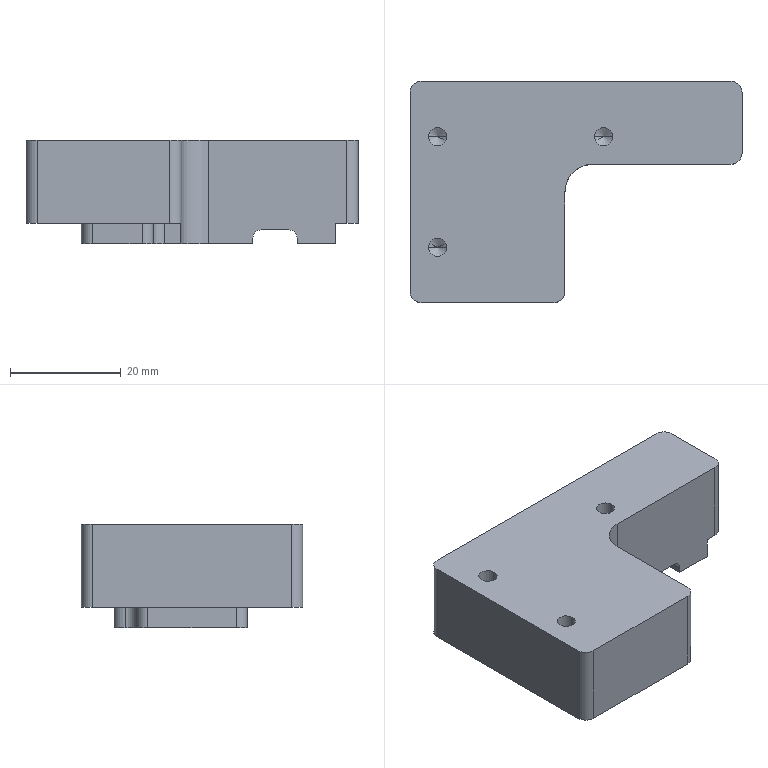Part | STEP file | 05-07-a pre-press block | 1 solid | 48 faces | box 60 x 40 x 18.7 mm | volume 25800 mm3 | cylinder 21 | plane 21 | cone 6 | commonest cylinder face diameters 4 x12 3.3 x6 3 x2 10 x1
STEP:
#1=CARTESIAN_POINT('',(-16.65,-10.,8.5));
#2=VERTEX_POINT('',#1);
#3=CARTESIAN_POINT('',(-13.35,-10.,8.5));
#4=VERTEX_POINT('',#3);
#5=CARTESIAN_POINT('',(-15.,-10.,8.5));
#6=DIRECTION('',(0.,0.,1.));
#7=DIRECTION('',(1.,0.,0.));
#8=AXIS2_PLACEMENT_3D('',#5,#6,#7);
#9=CIRCLE('',#8,1.65);
#10=EDGE_CURVE('',#2,#4,#9,.T.);
#11=ORIENTED_EDGE('',*,*,#10,.F.);
#12=CARTESIAN_POINT('',(-16.65,-10.,20.));
#13=VERTEX_POINT('',#12);
#14=CARTESIAN_POINT('',(-16.65,-10.,20.));
#15=DIRECTION('',(0.,0.,1.));
#16=VECTOR('',#15,1000.);
#17=LINE('',#14,#16);
#18=EDGE_CURVE('',#2,#13,#17,.T.);
#19=ORIENTED_EDGE('',*,*,#18,.T.);
#20=CARTESIAN_POINT('',(-13.35,-10.,20.));
#21=VERTEX_POINT('',#20);
#22=CARTESIAN_POINT('',(-15.,-10.,20.));
#23=DIRECTION('',(0.,0.,1.));
#24=DIRECTION('',(1.,0.,0.));
#25=AXIS2_PLACEMENT_3D('',#22,#23,#24);
#26=CIRCLE('',#25,1.65);
#27=EDGE_CURVE('',#13,#21,#26,.T.);
#28=ORIENTED_EDGE('',*,*,#27,.T.);
#29=CARTESIAN_POINT('',(-13.35,-10.,20.));
#30=DIRECTION('',(0.,0.,1.));
#31=VECTOR('',#30,1000.);
#32=LINE('',#29,#31);
#33=EDGE_CURVE('',#4,#21,#32,.T.);
#34=ORIENTED_EDGE('',*,*,#33,.F.);
#35=EDGE_LOOP('',(#11,#19,#28,#34));
#36=FACE_OUTER_BOUND('',#35,.T.);
#37=CARTESIAN_POINT('',(-15.,-10.,20.));
#38=DIRECTION('',(0.,0.,1.));
#39=DIRECTION('',(1.,0.,0.));
#40=AXIS2_PLACEMENT_3D('',#37,#38,#39);
#41=CYLINDRICAL_SURFACE('',#40,1.65);
#42=ADVANCED_FACE('',(#36),#41,.F.);
#43=CARTESIAN_POINT('',(-15.,-10.,7.509));
#44=VERTEX_POINT('',#43);
#45=CARTESIAN_POINT('',(-13.35,-10.,8.5));
#46=DIRECTION('',(0.8572,0.,0.515));
#47=VECTOR('',#46,1000.);
#48=LINE('',#45,#47);
#49=EDGE_CURVE('',#44,#4,#48,.T.);
#50=ORIENTED_EDGE('',*,*,#49,.F.);
#51=CARTESIAN_POINT('',(-16.65,-10.,8.5));
#52=DIRECTION('',(-0.8572,0.,0.515));
#53=VECTOR('',#52,1000.);
#54=LINE('',#51,#53);
#55=EDGE_CURVE('',#44,#2,#54,.T.);
#56=ORIENTED_EDGE('',*,*,#55,.T.);
#57=ORIENTED_EDGE('',*,*,#10,.T.);
#58=EDGE_LOOP('',(#50,#56,#57));
#59=FACE_OUTER_BOUND('',#58,.T.);
#60=CARTESIAN_POINT('',(-15.,-10.,8.5));
#61=DIRECTION('',(0.,0.,1.));
#62=DIRECTION('',(1.,0.,0.));
#63=AXIS2_PLACEMENT_3D('',#60,#61,#62);
#64=CONICAL_SURFACE('',#63,1.65,1.03);
#65=ADVANCED_FACE('',(#59),#64,.F.);
#66=CARTESIAN_POINT('',(13.35,10.,8.5));
#67=VERTEX_POINT('',#66);
#68=CARTESIAN_POINT('',(16.65,10.,8.5));
#69=VERTEX_POINT('',#68);
#70=CARTESIAN_POINT('',(15.,10.,8.5));
#71=DIRECTION('',(0.,0.,1.));
#72=DIRECTION('',(1.,0.,0.));
#73=AXIS2_PLACEMENT_3D('',#70,#71,#72);
#74=CIRCLE('',#73,1.65);
#75=EDGE_CURVE('',#67,#69,#74,.T.);
#76=ORIENTED_EDGE('',*,*,#75,.F.);
#77=CARTESIAN_POINT('',(13.35,10.,20.));
#78=VERTEX_POINT('',#77);
#79=CARTESIAN_POINT('',(13.35,10.,20.));
#80=DIRECTION('',(0.,0.,1.));
#81=VECTOR('',#80,1000.);
#82=LINE('',#79,#81);
#83=EDGE_CURVE('',#67,#78,#82,.T.);
#84=ORIENTED_EDGE('',*,*,#83,.T.);
#85=CARTESIAN_POINT('',(16.65,10.,20.));
#86=VERTEX_POINT('',#85);
#87=CARTESIAN_POINT('',(15.,10.,20.));
#88=DIRECTION('',(0.,0.,1.));
#89=DIRECTION('',(1.,0.,0.));
#90=AXIS2_PLACEMENT_3D('',#87,#88,#89);
#91=CIRCLE('',#90,1.65);
#92=EDGE_CURVE('',#78,#86,#91,.T.);
#93=ORIENTED_EDGE('',*,*,#92,.T.);
#94=CARTESIAN_POINT('',(16.65,10.,20.));
#95=DIRECTION('',(0.,0.,1.));
#96=VECTOR('',#95,1000.);
#97=LINE('',#94,#96);
#98=EDGE_CURVE('',#69,#86,#97,.T.);
#99=ORIENTED_EDGE('',*,*,#98,.F.);
#100=EDGE_LOOP('',(#76,#84,#93,#99));
#101=FACE_OUTER_BOUND('',#100,.T.);
#102=CARTESIAN_POINT('',(15.,10.,20.));
#103=DIRECTION('',(0.,0.,1.));
#104=DIRECTION('',(1.,0.,0.));
#105=AXIS2_PLACEMENT_3D('',#102,#103,#104);
#106=CYLINDRICAL_SURFACE('',#105,1.65);
#107=ADVANCED_FACE('',(#101),#106,.F.);
#108=CARTESIAN_POINT('',(15.,10.,7.509));
#109=VERTEX_POINT('',#108);
#110=CARTESIAN_POINT('',(16.65,10.,8.5));
#111=DIRECTION('',(0.8572,0.,0.515));
#112=VECTOR('',#111,1000.);
#113=LINE('',#110,#112);
#114=EDGE_CURVE('',#109,#69,#113,.T.);
#115=ORIENTED_EDGE('',*,*,#114,.F.);
#116=CARTESIAN_POINT('',(13.35,10.,8.5));
#117=DIRECTION('',(-0.8572,0.,0.515));
#118=VECTOR('',#117,1000.);
#119=LINE('',#116,#118);
#120=EDGE_CURVE('',#109,#67,#119,.T.);
#121=ORIENTED_EDGE('',*,*,#120,.T.);
#122=ORIENTED_EDGE('',*,*,#75,.T.);
#123=EDGE_LOOP('',(#115,#121,#122));
#124=FACE_OUTER_BOUND('',#123,.T.);
#125=CARTESIAN_POINT('',(15.,10.,8.5));
#126=DIRECTION('',(0.,0.,1.));
#127=DIRECTION('',(1.,0.,0.));
#128=AXIS2_PLACEMENT_3D('',#125,#126,#127);
#129=CONICAL_SURFACE('',#128,1.65,1.03);
#130=ADVANCED_FACE('',(#124),#129,.F.);
#131=CARTESIAN_POINT('',(-16.65,10.,8.5));
#132=VERTEX_POINT('',#131);
#133=CARTESIAN_POINT('',(-13.35,10.,8.5));
#134=VERTEX_POINT('',#133);
#135=CARTESIAN_POINT('',(-15.,10.,8.5));
#136=DIRECTION('',(0.,0.,1.));
#137=DIRECTION('',(1.,0.,0.));
#138=AXIS2_PLACEMENT_3D('',#135,#136,#137);
#139=CIRCLE('',#138,1.65);
#140=EDGE_CURVE('',#132,#134,#139,.T.);
#141=ORIENTED_EDGE('',*,*,#140,.F.);
#142=CARTESIAN_POINT('',(-16.65,10.,20.));
#143=VERTEX_POINT('',#142);
#144=CARTESIAN_POINT('',(-16.65,10.,20.));
#145=DIRECTION('',(0.,0.,1.));
#146=VECTOR('',#145,1000.);
#147=LINE('',#144,#146);
#148=EDGE_CURVE('',#132,#143,#147,.T.);
#149=ORIENTED_EDGE('',*,*,#148,.T.);
#150=CARTESIAN_POINT('',(-13.35,10.,20.));
#151=VERTEX_POINT('',#150);
#152=CARTESIAN_POINT('',(-15.,10.,20.));
#153=DIRECTION('',(0.,0.,1.));
#154=DIRECTION('',(1.,0.,0.));
#155=AXIS2_PLACEMENT_3D('',#152,#153,#154);
#156=CIRCLE('',#155,1.65);
#157=EDGE_CURVE('',#143,#151,#156,.T.);
#158=ORIENTED_EDGE('',*,*,#157,.T.);
#159=CARTESIAN_POINT('',(-13.35,10.,20.));
#160=DIRECTION('',(0.,0.,1.));
#161=VECTOR('',#160,1000.);
#162=LINE('',#159,#161);
#163=EDGE_CURVE('',#134,#151,#162,.T.);
#164=ORIENTED_EDGE('',*,*,#163,.F.);
#165=EDGE_LOOP('',(#141,#149,#158,#164));
#166=FACE_OUTER_BOUND('',#165,.T.);
#167=CARTESIAN_POINT('',(-15.,10.,20.));
#168=DIRECTION('',(0.,0.,1.));
#169=DIRECTION('',(1.,0.,0.));
#170=AXIS2_PLACEMENT_3D('',#167,#168,#169);
#171=CYLINDRICAL_SURFACE('',#170,1.65);
#172=ADVANCED_FACE('',(#166),#171,.F.);
#173=CARTESIAN_POINT('',(-15.,10.,7.509));
#174=VERTEX_POINT('',#173);
#175=CARTESIAN_POINT('',(-13.35,10.,8.5));
#176=DIRECTION('',(0.8572,0.,0.515));
#177=VECTOR('',#176,1000.);
#178=LINE('',#175,#177);
#179=EDGE_CURVE('',#174,#134,#178,.T.);
#180=ORIENTED_EDGE('',*,*,#179,.F.);
#181=CARTESIAN_POINT('',(-16.65,10.,8.5));
#182=DIRECTION('',(-0.8572,0.,0.515));
#183=VECTOR('',#182,1000.);
#184=LINE('',#181,#183);
#185=EDGE_CURVE('',#174,#132,#184,.T.);
#186=ORIENTED_EDGE('',*,*,#185,.T.);
#187=ORIENTED_EDGE('',*,*,#140,.T.);
#188=EDGE_LOOP('',(#180,#186,#187));
#189=FACE_OUTER_BOUND('',#188,.T.);
#190=CARTESIAN_POINT('',(-15.,10.,8.5));
#191=DIRECTION('',(0.,0.,1.));
#192=DIRECTION('',(1.,0.,0.));
#193=AXIS2_PLACEMENT_3D('',#190,#191,#192);
#194=CONICAL_SURFACE('',#193,1.65,1.03);
#195=ADVANCED_FACE('',(#189),#194,.F.);
#196=CARTESIAN_POINT('',(3.,-7.5,1.3));
#197=VERTEX_POINT('',#196);
#198=CARTESIAN_POINT('',(3.,-8.,1.3));
#199=VERTEX_POINT('',#198);
#200=CARTESIAN_POINT('',(3.,26.,1.3));
#201=DIRECTION('',(0.,-1.,0.));
#202=VECTOR('',#201,1000.);
#203=LINE('',#200,#202);
#204=EDGE_CURVE('',#197,#199,#203,.T.);
#205=ORIENTED_EDGE('',*,*,#204,.F.);
#206=CARTESIAN_POINT('',(3.,-7.5,5.));
#207=VERTEX_POINT('',#206);
#208=CARTESIAN_POINT('',(3.,-7.5,5.));
#209=DIRECTION('',(0.,0.,1.));
#210=VECTOR('',#209,1000.);
#211=LINE('',#208,#210);
#212=EDGE_CURVE('',#197,#207,#211,.T.);
#213=ORIENTED_EDGE('',*,*,#212,.T.);
#214=CARTESIAN_POINT('',(3.,-8.,5.));
#215=VERTEX_POINT('',#214);
#216=CARTESIAN_POINT('',(3.,-5.5,5.));
#217=DIRECTION('',(0.,1.,0.));
#218=VECTOR('',#217,1000.);
#219=LINE('',#216,#218);
#220=EDGE_CURVE('',#215,#207,#219,.T.);
#221=ORIENTED_EDGE('',*,*,#220,.F.);
#222=CARTESIAN_POINT('',(3.,-8.,1.3));
#223=DIRECTION('',(0.,0.,-1.));
#224=VECTOR('',#223,1000.);
#225=LINE('',#222,#224);
#226=EDGE_CURVE('',#215,#199,#225,.T.);
#227=ORIENTED_EDGE('',*,*,#226,.T.);
#228=EDGE_LOOP('',(#205,#213,#221,#227));
#229=FACE_OUTER_BOUND('',#228,.T.);
#230=CARTESIAN_POINT('',(3.,26.,1.3));
#231=DIRECTION('',(-1.,0.,0.));
#232=DIRECTION('',(0.,0.,1.));
#233=AXIS2_PLACEMENT_3D('',#230,#231,#232);
#234=PLANE('',#233);
#235=ADVANCED_FACE('',(#229),#234,.F.);
#236=CARTESIAN_POINT('',(-8.,10.,1.3));
#237=VERTEX_POINT('',#236);
#238=CARTESIAN_POINT('',(2.093,10.,1.3));
#239=VERTEX_POINT('',#238);
#240=CARTESIAN_POINT('',(4.093,10.,1.3));
#241=DIRECTION('',(1.,0.,0.));
#242=VECTOR('',#241,1000.);
#243=LINE('',#240,#242);
#244=EDGE_CURVE('',#237,#239,#243,.T.);
#245=ORIENTED_EDGE('',*,*,#244,.F.);
#246=CARTESIAN_POINT('',(-8.,10.,5.));
#247=VERTEX_POINT('',#246);
#248=CARTESIAN_POINT('',(-8.,10.,5.));
#249=DIRECTION('',(0.,0.,1.));
#250=VECTOR('',#249,1000.);
#251=LINE('',#248,#250);
#252=EDGE_CURVE('',#237,#247,#251,.T.);
#253=ORIENTED_EDGE('',*,*,#252,.T.);
#254=CARTESIAN_POINT('',(2.093,10.,5.));
#255=VERTEX_POINT('',#254);
#256=CARTESIAN_POINT('',(4.093,10.,5.));
#257=DIRECTION('',(-1.,0.,0.));
#258=VECTOR('',#257,1000.);
#259=LINE('',#256,#258);
#260=EDGE_CURVE('',#255,#247,#259,.T.);
#261=ORIENTED_EDGE('',*,*,#260,.F.);
#262=CARTESIAN_POINT('',(2.093,10.,1.3));
#263=DIRECTION('',(0.,0.,-1.));
#264=VECTOR('',#263,1000.);
#265=LINE('',#262,#264);
#266=EDGE_CURVE('',#255,#239,#265,.T.);
#267=ORIENTED_EDGE('',*,*,#266,.T.);
#268=EDGE_LOOP('',(#245,#253,#261,#267));
#269=FACE_OUTER_BOUND('',#268,.T.);
#270=CARTESIAN_POINT('',(4.093,10.,5.));
#271=DIRECTION('',(0.,-1.,0.));
#272=DIRECTION('',(0.,0.,-1.));
#273=AXIS2_PLACEMENT_3D('',#270,#271,#272);
#274=PLANE('',#273);
#275=ADVANCED_FACE('',(#269),#274,.F.);
#276=CARTESIAN_POINT('',(1.,-10.,1.3));
#277=VERTEX_POINT('',#276);
#278=CARTESIAN_POINT('',(-8.,-10.,1.3));
#279=VERTEX_POINT('',#278);
#280=CARTESIAN_POINT('',(3.,-10.,1.3));
#281=DIRECTION('',(-1.,0.,0.));
#282=VECTOR('',#281,1000.);
#283=LINE('',#280,#282);
#284=EDGE_CURVE('',#277,#279,#283,.T.);
#285=ORIENTED_EDGE('',*,*,#284,.F.);
#286=CARTESIAN_POINT('',(1.,-10.,5.));
#287=VERTEX_POINT('',#286);
#288=CARTESIAN_POINT('',(1.,-10.,5.));
#289=DIRECTION('',(0.,0.,1.));
#290=VECTOR('',#289,1000.);
#291=LINE('',#288,#290);
#292=EDGE_CURVE('',#277,#287,#291,.T.);
#293=ORIENTED_EDGE('',*,*,#292,.T.);
#294=CARTESIAN_POINT('',(-8.,-10.,5.));
#295=VERTEX_POINT('',#294);
#296=CARTESIAN_POINT('',(3.,-10.,5.));
#297=DIRECTION('',(1.,0.,0.));
#298=VECTOR('',#297,1000.);
#299=LINE('',#296,#298);
#300=EDGE_CURVE('',#295,#287,#299,.T.);
#301=ORIENTED_EDGE('',*,*,#300,.F.);
#302=CARTESIAN_POINT('',(-8.,-10.,5.));
#303=DIRECTION('',(0.,0.,-1.));
#304=VECTOR('',#303,1000.);
#305=LINE('',#302,#304);
#306=EDGE_CURVE('',#295,#279,#305,.T.);
#307=ORIENTED_EDGE('',*,*,#306,.T.);
#308=EDGE_LOOP('',(#285,#293,#301,#307));
#309=FACE_OUTER_BOUND('',#308,.T.);
#310=CARTESIAN_POINT('',(3.,-10.,5.));
#311=DIRECTION('',(0.,1.,0.));
#312=DIRECTION('',(-1.,0.,0.));
#313=AXIS2_PLACEMENT_3D('',#310,#311,#312);
#314=PLANE('',#313);
#315=ADVANCED_FACE('',(#309),#314,.F.);
#316=CARTESIAN_POINT('',(-10.,-8.,1.3));
#317=VERTEX_POINT('',#316);
#318=CARTESIAN_POINT('',(-10.,8.,1.3));
#319=VERTEX_POINT('',#318);
#320=CARTESIAN_POINT('',(-10.,10.,1.3));
#321=DIRECTION('',(0.,1.,0.));
#322=VECTOR('',#321,1000.);
#323=LINE('',#320,#322);
#324=EDGE_CURVE('',#317,#319,#323,.T.);
#325=ORIENTED_EDGE('',*,*,#324,.F.);
#326=CARTESIAN_POINT('',(-10.,-8.,5.));
#327=VERTEX_POINT('',#326);
#328=CARTESIAN_POINT('',(-10.,-8.,5.));
#329=DIRECTION('',(0.,0.,1.));
#330=VECTOR('',#329,1000.);
#331=LINE('',#328,#330);
#332=EDGE_CURVE('',#317,#327,#331,.T.);
#333=ORIENTED_EDGE('',*,*,#332,.T.);
#334=CARTESIAN_POINT('',(-10.,8.,5.));
#335=VERTEX_POINT('',#334);
#336=CARTESIAN_POINT('',(-10.,10.,5.));
#337=DIRECTION('',(0.,-1.,0.));
#338=VECTOR('',#337,1000.);
#339=LINE('',#336,#338);
#340=EDGE_CURVE('',#335,#327,#339,.T.);
#341=ORIENTED_EDGE('',*,*,#340,.F.);
#342=CARTESIAN_POINT('',(-10.,8.,5.));
#343=DIRECTION('',(0.,0.,-1.));
#344=VECTOR('',#343,1000.);
#345=LINE('',#342,#344);
#346=EDGE_CURVE('',#335,#319,#345,.T.);
#347=ORIENTED_EDGE('',*,*,#346,.T.);
#348=EDGE_LOOP('',(#325,#333,#341,#347));
#349=FACE_OUTER_BOUND('',#348,.T.);
#350=CARTESIAN_POINT('',(-10.,10.,5.));
#351=DIRECTION('',(1.,0.,0.));
#352=DIRECTION('',(0.,1.,0.));
#353=AXIS2_PLACEMENT_3D('',#350,#351,#352);
#354=PLANE('',#353);
#355=ADVANCED_FACE('',(#349),#354,.F.);
#356=ORIENTED_EDGE('',*,*,#252,.F.);
#357=CARTESIAN_POINT('',(-8.,8.,1.3));
#358=DIRECTION('',(0.,0.,1.));
#359=DIRECTION('',(-1.,0.,0.));
#360=AXIS2_PLACEMENT_3D('',#357,#358,#359);
#361=CIRCLE('',#360,2.);
#362=EDGE_CURVE('',#237,#319,#361,.T.);
#363=ORIENTED_EDGE('',*,*,#362,.T.);
#364=ORIENTED_EDGE('',*,*,#346,.F.);
#365=CARTESIAN_POINT('',(-8.,8.,5.));
#366=DIRECTION('',(0.,0.,1.));
#367=DIRECTION('',(-1.,0.,0.));
#368=AXIS2_PLACEMENT_3D('',#365,#366,#367);
#369=CIRCLE('',#368,2.);
#370=EDGE_CURVE('',#247,#335,#369,.T.);
#371=ORIENTED_EDGE('',*,*,#370,.F.);
#372=EDGE_LOOP('',(#356,#363,#364,#371));
#373=FACE_OUTER_BOUND('',#372,.T.);
#374=CARTESIAN_POINT('',(-8.,8.,5.));
#375=DIRECTION('',(0.,0.,-1.));
#376=DIRECTION('',(-1.,0.,0.));
#377=AXIS2_PLACEMENT_3D('',#374,#375,#376);
#378=CYLINDRICAL_SURFACE('',#377,2.);
#379=ADVANCED_FACE('',(#373),#378,.T.);
#380=ORIENTED_EDGE('',*,*,#332,.F.);
#381=CARTESIAN_POINT('',(-8.,-8.,1.3));
#382=DIRECTION('',(0.,0.,1.));
#383=DIRECTION('',(-1.,0.,0.));
#384=AXIS2_PLACEMENT_3D('',#381,#382,#383);
#385=CIRCLE('',#384,2.);
#386=EDGE_CURVE('',#317,#279,#385,.T.);
#387=ORIENTED_EDGE('',*,*,#386,.T.);
#388=ORIENTED_EDGE('',*,*,#306,.F.);
#389=CARTESIAN_POINT('',(-8.,-8.,5.));
#390=DIRECTION('',(0.,0.,1.));
#391=DIRECTION('',(-1.,0.,0.));
#392=AXIS2_PLACEMENT_3D('',#389,#390,#391);
#393=CIRCLE('',#392,2.);
#394=EDGE_CURVE('',#327,#295,#393,.T.);
#395=ORIENTED_EDGE('',*,*,#394,.F.);
#396=EDGE_LOOP('',(#380,#387,#388,#395));
#397=FACE_OUTER_BOUND('',#396,.T.);
#398=CARTESIAN_POINT('',(-8.,-8.,5.));
#399=DIRECTION('',(0.,0.,-1.));
#400=DIRECTION('',(-1.,0.,0.));
#401=AXIS2_PLACEMENT_3D('',#398,#399,#400);
#402=CYLINDRICAL_SURFACE('',#401,2.);
#403=ADVANCED_FACE('',(#397),#402,.T.);
#404=ORIENTED_EDGE('',*,*,#292,.F.);
#405=CARTESIAN_POINT('',(1.,-8.,1.3));
#406=DIRECTION('',(0.,0.,1.));
#407=DIRECTION('',(-1.,0.,0.));
#408=AXIS2_PLACEMENT_3D('',#405,#406,#407);
#409=CIRCLE('',#408,2.);
#410=EDGE_CURVE('',#277,#199,#409,.T.);
#411=ORIENTED_EDGE('',*,*,#410,.T.);
#412=ORIENTED_EDGE('',*,*,#226,.F.);
#413=CARTESIAN_POINT('',(1.,-8.,5.));
#414=DIRECTION('',(0.,0.,1.));
#415=DIRECTION('',(-1.,0.,0.));
#416=AXIS2_PLACEMENT_3D('',#413,#414,#415);
#417=CIRCLE('',#416,2.);
#418=EDGE_CURVE('',#287,#215,#417,.T.);
#419=ORIENTED_EDGE('',*,*,#418,.F.);
#420=EDGE_LOOP('',(#404,#411,#412,#419));
#421=FACE_OUTER_BOUND('',#420,.T.);
#422=CARTESIAN_POINT('',(1.,-8.,1.3));
#423=DIRECTION('',(0.,0.,-1.));
#424=DIRECTION('',(-1.,0.,0.));
#425=AXIS2_PLACEMENT_3D('',#422,#423,#424);
#426=CYLINDRICAL_SURFACE('',#425,2.);
#427=ADVANCED_FACE('',(#421),#426,.T.);
#428=CARTESIAN_POINT('',(4.093,12.,1.3));
#429=VERTEX_POINT('',#428);
#430=CARTESIAN_POINT('',(2.093,12.,1.3));
#431=DIRECTION('',(0.,0.,1.));
#432=DIRECTION('',(1.,0.,0.));
#433=AXIS2_PLACEMENT_3D('',#430,#431,#432);
#434=CIRCLE('',#433,2.);
#435=EDGE_CURVE('',#239,#429,#434,.T.);
#436=ORIENTED_EDGE('',*,*,#435,.F.);
#437=ORIENTED_EDGE('',*,*,#266,.F.);
#438=CARTESIAN_POINT('',(4.093,12.,5.));
#439=VERTEX_POINT('',#438);
#440=CARTESIAN_POINT('',(2.093,12.,5.));
#441=DIRECTION('',(0.,0.,-1.));
#442=DIRECTION('',(-1.,0.,0.));
#443=AXIS2_PLACEMENT_3D('',#440,#441,#442);
#444=CIRCLE('',#443,2.);
#445=EDGE_CURVE('',#439,#255,#444,.T.);
#446=ORIENTED_EDGE('',*,*,#445,.F.);
#447=CARTESIAN_POINT('',(4.093,12.,5.));
#448=DIRECTION('',(0.,0.,1.));
#449=VECTOR('',#448,1000.);
#450=LINE('',#447,#449);
#451=EDGE_CURVE('',#429,#439,#450,.T.);
#452=ORIENTED_EDGE('',*,*,#451,.F.);
#453=EDGE_LOOP('',(#436,#437,#446,#452));
#454=FACE_OUTER_BOUND('',#453,.T.);
#455=CARTESIAN_POINT('',(2.093,12.,5.));
#456=DIRECTION('',(0.,0.,1.));
#457=DIRECTION('',(1.,0.,0.));
#458=AXIS2_PLACEMENT_3D('',#455,#456,#457);
#459=CYLINDRICAL_SURFACE('',#458,2.);
#460=ADVANCED_FACE('',(#454),#459,.F.);
#461=CARTESIAN_POINT('',(4.093,12.096,1.3));
#462=VERTEX_POINT('',#461);
#463=CARTESIAN_POINT('',(6.093,14.096,1.3));
#464=VERTEX_POINT('',#463);
#465=CARTESIAN_POINT('',(6.093,12.096,1.3));
#466=DIRECTION('',(0.,0.,-1.));
#467=DIRECTION('',(1.,0.,0.));
#468=AXIS2_PLACEMENT_3D('',#465,#466,#467);
#469=CIRCLE('',#468,2.);
#470=EDGE_CURVE('',#462,#464,#469,.T.);
#471=ORIENTED_EDGE('',*,*,#470,.T.);
#472=CARTESIAN_POINT('',(21.01,14.096,1.3));
#473=VERTEX_POINT('',#472);
#474=CARTESIAN_POINT('',(20.,14.096,1.3));
#475=DIRECTION('',(1.,0.,0.));
#476=VECTOR('',#475,1000.);
#477=LINE('',#474,#476);
#478=EDGE_CURVE('',#464,#473,#477,.T.);
#479=ORIENTED_EDGE('',*,*,#478,.T.);
#480=CARTESIAN_POINT('',(21.01,5.,1.3));
#481=VERTEX_POINT('',#480);
#482=CARTESIAN_POINT('',(21.01,26.,1.3));
#483=DIRECTION('',(0.,-1.,0.));
#484=VECTOR('',#483,1000.);
#485=LINE('',#482,#484);
#486=EDGE_CURVE('',#473,#481,#485,.T.);
#487=ORIENTED_EDGE('',*,*,#486,.T.);
#488=CARTESIAN_POINT('',(13.,5.,1.3));
#489=VERTEX_POINT('',#488);
#490=CARTESIAN_POINT('',(20.,5.,1.3));
#491=DIRECTION('',(-1.,0.,0.));
#492=VECTOR('',#491,1000.);
#493=LINE('',#490,#492);
#494=EDGE_CURVE('',#481,#489,#493,.T.);
#495=ORIENTED_EDGE('',*,*,#494,.T.);
#496=CARTESIAN_POINT('',(8.,0.,1.3));
#497=VERTEX_POINT('',#496);
#498=CARTESIAN_POINT('',(13.,0.,1.3));
#499=DIRECTION('',(0.,0.,1.));
#500=DIRECTION('',(1.,0.,0.));
#501=AXIS2_PLACEMENT_3D('',#498,#499,#500);
#502=CIRCLE('',#501,5.);
#503=EDGE_CURVE('',#489,#497,#502,.T.);
#504=ORIENTED_EDGE('',*,*,#503,.T.);
#505=CARTESIAN_POINT('',(8.,-5.5,1.3));
#506=VERTEX_POINT('',#505);
#507=CARTESIAN_POINT('',(8.,26.,1.3));
#508=DIRECTION('',(0.,-1.,0.));
#509=VECTOR('',#508,1000.);
#510=LINE('',#507,#509);
#511=EDGE_CURVE('',#497,#506,#510,.T.);
#512=ORIENTED_EDGE('',*,*,#511,.T.);
#513=CARTESIAN_POINT('',(5.,-5.5,1.3));
#514=VERTEX_POINT('',#513);
#515=CARTESIAN_POINT('',(20.,-5.5,1.3));
#516=DIRECTION('',(-1.,0.,0.));
#517=VECTOR('',#516,1000.);
#518=LINE('',#515,#517);
#519=EDGE_CURVE('',#506,#514,#518,.T.);
#520=ORIENTED_EDGE('',*,*,#519,.T.);
#521=CARTESIAN_POINT('',(5.,-7.5,1.3));
#522=DIRECTION('',(0.,0.,1.));
#523=DIRECTION('',(1.,0.,0.));
#524=AXIS2_PLACEMENT_3D('',#521,#522,#523);
#525=CIRCLE('',#524,2.);
#526=EDGE_CURVE('',#514,#197,#525,.T.);
#527=ORIENTED_EDGE('',*,*,#526,.T.);
#528=ORIENTED_EDGE('',*,*,#204,.T.);
#529=ORIENTED_EDGE('',*,*,#410,.F.);
#530=ORIENTED_EDGE('',*,*,#284,.T.);
#531=ORIENTED_EDGE('',*,*,#386,.F.);
#532=ORIENTED_EDGE('',*,*,#324,.T.);
#533=ORIENTED_EDGE('',*,*,#362,.F.);
#534=ORIENTED_EDGE('',*,*,#244,.T.);
#535=ORIENTED_EDGE('',*,*,#435,.T.);
#536=CARTESIAN_POINT('',(4.093,26.,1.3));
#537=DIRECTION('',(0.,1.,0.));
#538=VECTOR('',#537,1000.);
#539=LINE('',#536,#538);
#540=EDGE_CURVE('',#429,#462,#539,.T.);
#541=ORIENTED_EDGE('',*,*,#540,.T.);
#542=EDGE_LOOP('',(#471,#479,#487,#495,#504,#512,#520,#527,#528,#529,#530,#531,#532,#533,#534,#535,#541));
#543=FACE_OUTER_BOUND('',#542,.T.);
#544=CARTESIAN_POINT('',(20.,26.,1.3));
#545=DIRECTION('',(0.,0.,1.));
#546=DIRECTION('',(1.,0.,0.));
#547=AXIS2_PLACEMENT_3D('',#544,#545,#546);
#548=PLANE('',#547);
#549=ADVANCED_FACE('',(#543),#548,.F.);
#550=CARTESIAN_POINT('',(38.,5.,5.));
#551=VERTEX_POINT('',#550);
#552=CARTESIAN_POINT('',(36.,5.,5.));
#553=VERTEX_POINT('',#552);
#554=CARTESIAN_POINT('',(18.,5.,5.));
#555=DIRECTION('',(-1.,0.,0.));
#556=VECTOR('',#555,1000.);
#557=LINE('',#554,#556);
#558=EDGE_CURVE('',#551,#553,#557,.T.);
#559=ORIENTED_EDGE('',*,*,#558,.T.);
#560=CARTESIAN_POINT('',(36.,12.096,5.));
#561=VERTEX_POINT('',#560);
#562=CARTESIAN_POINT('',(36.,12.096,5.));
#563=DIRECTION('',(0.,-1.,0.));
#564=VECTOR('',#563,1000.);
#565=LINE('',#562,#564);
#566=EDGE_CURVE('',#561,#553,#565,.T.);
#567=ORIENTED_EDGE('',*,*,#566,.F.);
#568=CARTESIAN_POINT('',(34.,14.096,5.));
#569=VERTEX_POINT('',#568);
#570=CARTESIAN_POINT('',(34.,12.096,5.));
#571=DIRECTION('',(0.,0.,-1.));
#572=DIRECTION('',(1.,0.,0.));
#573=AXIS2_PLACEMENT_3D('',#570,#571,#572);
#574=CIRCLE('',#573,2.);
#575=EDGE_CURVE('',#569,#561,#574,.T.);
#576=ORIENTED_EDGE('',*,*,#575,.F.);
#577=CARTESIAN_POINT('',(6.093,14.096,5.));
#578=VERTEX_POINT('',#577);
#579=CARTESIAN_POINT('',(20.,14.096,5.));
#580=DIRECTION('',(-1.,0.,0.));
#581=VECTOR('',#580,1000.);
#582=LINE('',#579,#581);
#583=EDGE_CURVE('',#569,#578,#582,.T.);
#584=ORIENTED_EDGE('',*,*,#583,.T.);
#585=CARTESIAN_POINT('',(4.093,12.096,5.));
#586=VERTEX_POINT('',#585);
#587=CARTESIAN_POINT('',(6.093,12.096,5.));
#588=DIRECTION('',(0.,0.,1.));
#589=DIRECTION('',(-1.,0.,0.));
#590=AXIS2_PLACEMENT_3D('',#587,#588,#589);
#591=CIRCLE('',#590,2.);
#592=EDGE_CURVE('',#578,#586,#591,.T.);
#593=ORIENTED_EDGE('',*,*,#592,.T.);
#594=CARTESIAN_POINT('',(4.093,14.096,5.));
#595=DIRECTION('',(0.,-1.,0.));
#596=VECTOR('',#595,1000.);
#597=LINE('',#594,#596);
#598=EDGE_CURVE('',#586,#439,#597,.T.);
#599=ORIENTED_EDGE('',*,*,#598,.T.);
#600=ORIENTED_EDGE('',*,*,#445,.T.);
#601=ORIENTED_EDGE('',*,*,#260,.T.);
#602=ORIENTED_EDGE('',*,*,#370,.T.);
#603=ORIENTED_EDGE('',*,*,#340,.T.);
#604=ORIENTED_EDGE('',*,*,#394,.T.);
#605=ORIENTED_EDGE('',*,*,#300,.T.);
#606=ORIENTED_EDGE('',*,*,#418,.T.);
#607=ORIENTED_EDGE('',*,*,#220,.T.);
#608=CARTESIAN_POINT('',(5.,-5.5,5.));
#609=VERTEX_POINT('',#608);
#610=CARTESIAN_POINT('',(5.,-7.5,5.));
#611=DIRECTION('',(0.,0.,-1.));
#612=DIRECTION('',(-1.,0.,0.));
#613=AXIS2_PLACEMENT_3D('',#610,#611,#612);
#614=CIRCLE('',#613,2.);
#615=EDGE_CURVE('',#207,#609,#614,.T.);
#616=ORIENTED_EDGE('',*,*,#615,.T.);
#617=CARTESIAN_POINT('',(8.,-5.5,5.));
#618=VERTEX_POINT('',#617);
#619=CARTESIAN_POINT('',(20.,-5.5,5.));
#620=DIRECTION('',(1.,0.,0.));
#621=VECTOR('',#620,1000.);
#622=LINE('',#619,#621);
#623=EDGE_CURVE('',#609,#618,#622,.T.);
#624=ORIENTED_EDGE('',*,*,#623,.T.);
#625=CARTESIAN_POINT('',(8.,-18.,5.));
#626=VERTEX_POINT('',#625);
#627=CARTESIAN_POINT('',(8.,10.,5.));
#628=DIRECTION('',(0.,1.,0.));
#629=VECTOR('',#628,1000.);
#630=LINE('',#627,#629);
#631=EDGE_CURVE('',#626,#618,#630,.T.);
#632=ORIENTED_EDGE('',*,*,#631,.F.);
#633=CARTESIAN_POINT('',(6.,-20.,5.));
#634=VERTEX_POINT('',#633);
#635=CARTESIAN_POINT('',(6.,-18.,5.));
#636=DIRECTION('',(0.,0.,-1.));
#637=DIRECTION('',(-1.,0.,0.));
#638=AXIS2_PLACEMENT_3D('',#635,#636,#637);
#639=CIRCLE('',#638,2.);
#640=EDGE_CURVE('',#626,#634,#639,.T.);
#641=ORIENTED_EDGE('',*,*,#640,.T.);
#642=CARTESIAN_POINT('',(-18.,-20.,5.));
#643=VERTEX_POINT('',#642);
#644=CARTESIAN_POINT('',(-20.,-20.,5.));
#645=DIRECTION('',(-1.,0.,0.));
#646=VECTOR('',#645,1000.);
#647=LINE('',#644,#646);
#648=EDGE_CURVE('',#634,#643,#647,.T.);
#649=ORIENTED_EDGE('',*,*,#648,.T.);
#650=CARTESIAN_POINT('',(-20.,-18.,5.));
#651=VERTEX_POINT('',#650);
#652=CARTESIAN_POINT('',(-18.,-18.,5.));
#653=DIRECTION('',(0.,0.,-1.));
#654=DIRECTION('',(-1.,0.,0.));
#655=AXIS2_PLACEMENT_3D('',#652,#653,#654);
#656=CIRCLE('',#655,2.);
#657=EDGE_CURVE('',#643,#651,#656,.T.);
#658=ORIENTED_EDGE('',*,*,#657,.T.);
#659=CARTESIAN_POINT('',(-20.,18.,5.));
#660=VERTEX_POINT('',#659);
#661=CARTESIAN_POINT('',(-20.,20.,5.));
#662=DIRECTION('',(0.,1.,0.));
#663=VECTOR('',#662,1000.);
#664=LINE('',#661,#663);
#665=EDGE_CURVE('',#651,#660,#664,.T.);
#666=ORIENTED_EDGE('',*,*,#665,.T.);
#667=CARTESIAN_POINT('',(-18.,20.,5.));
#668=VERTEX_POINT('',#667);
#669=CARTESIAN_POINT('',(-18.,18.,5.));
#670=DIRECTION('',(0.,0.,-1.));
#671=DIRECTION('',(-1.,0.,0.));
#672=AXIS2_PLACEMENT_3D('',#669,#670,#671);
#673=CIRCLE('',#672,2.);
#674=EDGE_CURVE('',#660,#668,#673,.T.);
#675=ORIENTED_EDGE('',*,*,#674,.T.);
#676=CARTESIAN_POINT('',(38.,20.,5.));
#677=VERTEX_POINT('',#676);
#678=CARTESIAN_POINT('',(-20.,20.,5.));
#679=DIRECTION('',(1.,0.,0.));
#680=VECTOR('',#679,1000.);
#681=LINE('',#678,#680);
#682=EDGE_CURVE('',#668,#677,#681,.T.);
#683=ORIENTED_EDGE('',*,*,#682,.T.);
#684=CARTESIAN_POINT('',(40.,18.,5.));
#685=VERTEX_POINT('',#684);
#686=CARTESIAN_POINT('',(38.,18.,5.));
#687=DIRECTION('',(0.,0.,-1.));
#688=DIRECTION('',(-1.,0.,0.));
#689=AXIS2_PLACEMENT_3D('',#686,#687,#688);
#690=CIRCLE('',#689,2.);
#691=EDGE_CURVE('',#677,#685,#690,.T.);
#692=ORIENTED_EDGE('',*,*,#691,.T.);
#693=CARTESIAN_POINT('',(40.,7.,5.));
#694=VERTEX_POINT('',#693);
#695=CARTESIAN_POINT('',(40.,20.,5.));
#696=DIRECTION('',(0.,-1.,0.));
#697=VECTOR('',#696,1000.);
#698=LINE('',#695,#697);
#699=EDGE_CURVE('',#685,#694,#698,.T.);
#700=ORIENTED_EDGE('',*,*,#699,.T.);
#701=CARTESIAN_POINT('',(38.,7.,5.));
#702=DIRECTION('',(0.,0.,-1.));
#703=DIRECTION('',(-1.,0.,0.));
#704=AXIS2_PLACEMENT_3D('',#701,#702,#703);
#705=CIRCLE('',#704,2.);
#706=EDGE_CURVE('',#694,#551,#705,.T.);
#707=ORIENTED_EDGE('',*,*,#706,.T.);
#708=EDGE_LOOP('',(#559,#567,#576,#584,#593,#599,#600,#601,#602,#603,#604,#605,#606,#607,#616,#624,#632,#641,#649,#658,#666,#675,#683,#692,#700,#707));
#709=FACE_OUTER_BOUND('',#708,.T.);
#710=CARTESIAN_POINT('',(4.093,10.,5.));
#711=DIRECTION('',(0.,0.,-1.));
#712=DIRECTION('',(-1.,0.,0.));
#713=AXIS2_PLACEMENT_3D('',#710,#711,#712);
#714=PLANE('',#713);
#715=ADVANCED_FACE('',(#709),#714,.T.);
#716=CARTESIAN_POINT('',(38.,20.,20.));
#717=VERTEX_POINT('',#716);
#718=CARTESIAN_POINT('',(-18.,20.,20.));
#719=VERTEX_POINT('',#718);
#720=CARTESIAN_POINT('',(-20.,20.,20.));
#721=DIRECTION('',(-1.,0.,0.));
#722=VECTOR('',#721,1000.);
#723=LINE('',#720,#722);
#724=EDGE_CURVE('',#717,#719,#723,.T.);
#725=ORIENTED_EDGE('',*,*,#724,.F.);
#726=CARTESIAN_POINT('',(38.,20.,5.));
#727=DIRECTION('',(0.,0.,-1.));
#728=VECTOR('',#727,1000.);
#729=LINE('',#726,#728);
#730=EDGE_CURVE('',#717,#677,#729,.T.);
#731=ORIENTED_EDGE('',*,*,#730,.T.);
#732=ORIENTED_EDGE('',*,*,#682,.F.);
#733=CARTESIAN_POINT('',(-18.,20.,20.));
#734=DIRECTION('',(0.,0.,1.));
#735=VECTOR('',#734,1000.);
#736=LINE('',#733,#735);
#737=EDGE_CURVE('',#668,#719,#736,.T.);
#738=ORIENTED_EDGE('',*,*,#737,.T.);
#739=EDGE_LOOP('',(#725,#731,#732,#738));
#740=FACE_OUTER_BOUND('',#739,.T.);
#741=CARTESIAN_POINT('',(-20.,20.,20.));
#742=DIRECTION('',(0.,-1.,0.));
#743=DIRECTION('',(0.,0.,-1.));
#744=AXIS2_PLACEMENT_3D('',#741,#742,#743);
#745=PLANE('',#744);
#746=ADVANCED_FACE('',(#740),#745,.F.);
#747=CARTESIAN_POINT('',(-20.,18.,20.));
#748=VERTEX_POINT('',#747);
#749=CARTESIAN_POINT('',(-20.,-18.,20.));
#750=VERTEX_POINT('',#749);
#751=CARTESIAN_POINT('',(-20.,20.,20.));
#752=DIRECTION('',(0.,-1.,0.));
#753=VECTOR('',#752,1000.);
#754=LINE('',#751,#753);
#755=EDGE_CURVE('',#748,#750,#754,.T.);
#756=ORIENTED_EDGE('',*,*,#755,.F.);
#757=CARTESIAN_POINT('',(-20.,18.,20.));
#758=DIRECTION('',(0.,0.,-1.));
#759=VECTOR('',#758,1000.);
#760=LINE('',#757,#759);
#761=EDGE_CURVE('',#748,#660,#760,.T.);
#762=ORIENTED_EDGE('',*,*,#761,.T.);
#763=ORIENTED_EDGE('',*,*,#665,.F.);
#764=CARTESIAN_POINT('',(-20.,-18.,20.));
#765=DIRECTION('',(0.,0.,1.));
#766=VECTOR('',#765,1000.);
#767=LINE('',#764,#766);
#768=EDGE_CURVE('',#651,#750,#767,.T.);
#769=ORIENTED_EDGE('',*,*,#768,.T.);
#770=EDGE_LOOP('',(#756,#762,#763,#769));
#771=FACE_OUTER_BOUND('',#770,.T.);
#772=CARTESIAN_POINT('',(-20.,20.,20.));
#773=DIRECTION('',(1.,0.,0.));
#774=DIRECTION('',(0.,1.,0.));
#775=AXIS2_PLACEMENT_3D('',#772,#773,#774);
#776=PLANE('',#775);
#777=ADVANCED_FACE('',(#771),#776,.F.);
#778=ORIENTED_EDGE('',*,*,#648,.F.);
#779=CARTESIAN_POINT('',(6.,-20.,20.));
#780=VERTEX_POINT('',#779);
#781=CARTESIAN_POINT('',(6.,-20.,20.));
#782=DIRECTION('',(0.,0.,1.));
#783=VECTOR('',#782,1000.);
#784=LINE('',#781,#783);
#785=EDGE_CURVE('',#634,#780,#784,.T.);
#786=ORIENTED_EDGE('',*,*,#785,.T.);
#787=CARTESIAN_POINT('',(-18.,-20.,20.));
#788=VERTEX_POINT('',#787);
#789=CARTESIAN_POINT('',(-20.,-20.,20.));
#790=DIRECTION('',(1.,0.,0.));
#791=VECTOR('',#790,1000.);
#792=LINE('',#789,#791);
#793=EDGE_CURVE('',#788,#780,#792,.T.);
#794=ORIENTED_EDGE('',*,*,#793,.F.);
#795=CARTESIAN_POINT('',(-18.,-20.,20.));
#796=DIRECTION('',(0.,0.,-1.));
#797=VECTOR('',#796,1000.);
#798=LINE('',#795,#797);
#799=EDGE_CURVE('',#788,#643,#798,.T.);
#800=ORIENTED_EDGE('',*,*,#799,.T.);
#801=EDGE_LOOP('',(#778,#786,#794,#800));
#802=FACE_OUTER_BOUND('',#801,.T.);
#803=CARTESIAN_POINT('',(-20.,-20.,20.));
#804=DIRECTION('',(0.,1.,0.));
#805=DIRECTION('',(0.,0.,1.));
#806=AXIS2_PLACEMENT_3D('',#803,#804,#805);
#807=PLANE('',#806);
#808=ADVANCED_FACE('',(#802),#807,.F.);
#809=CARTESIAN_POINT('',(40.,18.,20.));
#810=VERTEX_POINT('',#809);
#811=CARTESIAN_POINT('',(40.,7.,20.));
#812=VERTEX_POINT('',#811);
#813=CARTESIAN_POINT('',(40.,20.,20.));
#814=DIRECTION('',(0.,-1.,0.));
#815=VECTOR('',#814,1000.);
#816=LINE('',#813,#815);
#817=EDGE_CURVE('',#810,#812,#816,.T.);
#818=ORIENTED_EDGE('',*,*,#817,.F.);
#819=CARTESIAN_POINT('',(38.,18.,20.));
#820=DIRECTION('',(0.,0.,1.));
#821=DIRECTION('',(1.,0.,0.));
#822=AXIS2_PLACEMENT_3D('',#819,#820,#821);
#823=CIRCLE('',#822,2.);
#824=EDGE_CURVE('',#810,#717,#823,.T.);
#825=ORIENTED_EDGE('',*,*,#824,.T.);
#826=ORIENTED_EDGE('',*,*,#724,.T.);
#827=CARTESIAN_POINT('',(-18.,18.,20.));
#828=DIRECTION('',(0.,0.,1.));
#829=DIRECTION('',(1.,0.,0.));
#830=AXIS2_PLACEMENT_3D('',#827,#828,#829);
#831=CIRCLE('',#830,2.);
#832=EDGE_CURVE('',#719,#748,#831,.T.);
#833=ORIENTED_EDGE('',*,*,#832,.T.);
#834=ORIENTED_EDGE('',*,*,#755,.T.);
#835=CARTESIAN_POINT('',(-18.,-18.,20.));
#836=DIRECTION('',(0.,0.,1.));
#837=DIRECTION('',(1.,0.,0.));
#838=AXIS2_PLACEMENT_3D('',#835,#836,#837);
#839=CIRCLE('',#838,2.);
#840=EDGE_CURVE('',#750,#788,#839,.T.);
#841=ORIENTED_EDGE('',*,*,#840,.T.);
#842=ORIENTED_EDGE('',*,*,#793,.T.);
#843=CARTESIAN_POINT('',(8.,-18.,20.));
#844=VERTEX_POINT('',#843);
#845=CARTESIAN_POINT('',(6.,-18.,20.));
#846=DIRECTION('',(0.,0.,1.));
#847=DIRECTION('',(1.,0.,0.));
#848=AXIS2_PLACEMENT_3D('',#845,#846,#847);
#849=CIRCLE('',#848,2.);
#850=EDGE_CURVE('',#780,#844,#849,.T.);
#851=ORIENTED_EDGE('',*,*,#850,.T.);
#852=CARTESIAN_POINT('',(8.,0.,20.));
#853=VERTEX_POINT('',#852);
#854=CARTESIAN_POINT('',(8.,0.,20.));
#855=DIRECTION('',(0.,-1.,0.));
#856=VECTOR('',#855,1000.);
#857=LINE('',#854,#856);
#858=EDGE_CURVE('',#853,#844,#857,.T.);
#859=ORIENTED_EDGE('',*,*,#858,.F.);
#860=CARTESIAN_POINT('',(13.,5.,20.));
#861=VERTEX_POINT('',#860);
#862=CARTESIAN_POINT('',(13.,0.,20.));
#863=DIRECTION('',(0.,0.,1.));
#864=DIRECTION('',(-1.,0.,0.));
#865=AXIS2_PLACEMENT_3D('',#862,#863,#864);
#866=CIRCLE('',#865,5.);
#867=EDGE_CURVE('',#861,#853,#866,.T.);
#868=ORIENTED_EDGE('',*,*,#867,.F.);
#869=CARTESIAN_POINT('',(38.,5.,20.));
#870=VERTEX_POINT('',#869);
#871=CARTESIAN_POINT('',(31.615,5.,20.));
#872=DIRECTION('',(-1.,0.,0.));
#873=VECTOR('',#872,1000.);
#874=LINE('',#871,#873);
#875=EDGE_CURVE('',#870,#861,#874,.T.);
#876=ORIENTED_EDGE('',*,*,#875,.F.);
#877=CARTESIAN_POINT('',(38.,7.,20.));
#878=DIRECTION('',(0.,0.,1.));
#879=DIRECTION('',(1.,0.,0.));
#880=AXIS2_PLACEMENT_3D('',#877,#878,#879);
#881=CIRCLE('',#880,2.);
#882=EDGE_CURVE('',#870,#812,#881,.T.);
#883=ORIENTED_EDGE('',*,*,#882,.T.);
#884=EDGE_LOOP('',(#818,#825,#826,#833,#834,#841,#842,#851,#859,#868,#876,#883));
#885=FACE_OUTER_BOUND('',#884,.T.);
#886=CARTESIAN_POINT('',(-15.,-10.,20.));
#887=DIRECTION('',(0.,0.,1.));
#888=DIRECTION('',(1.,0.,0.));
#889=AXIS2_PLACEMENT_3D('',#886,#887,#888);
#890=CIRCLE('',#889,1.65);
#891=EDGE_CURVE('',#21,#13,#890,.T.);
#892=ORIENTED_EDGE('',*,*,#891,.F.);
#893=ORIENTED_EDGE('',*,*,#27,.F.);
#894=EDGE_LOOP('',(#892,#893));
#895=FACE_BOUND('',#894,.T.);
#896=CARTESIAN_POINT('',(15.,10.,20.));
#897=DIRECTION('',(0.,0.,1.));
#898=DIRECTION('',(1.,0.,0.));
#899=AXIS2_PLACEMENT_3D('',#896,#897,#898);
#900=CIRCLE('',#899,1.65);
#901=EDGE_CURVE('',#86,#78,#900,.T.);
#902=ORIENTED_EDGE('',*,*,#901,.F.);
#903=ORIENTED_EDGE('',*,*,#92,.F.);
#904=EDGE_LOOP('',(#902,#903));
#905=FACE_BOUND('',#904,.T.);
#906=CARTESIAN_POINT('',(-15.,10.,20.));
#907=DIRECTION('',(0.,0.,1.));
#908=DIRECTION('',(1.,0.,0.));
#909=AXIS2_PLACEMENT_3D('',#906,#907,#908);
#910=CIRCLE('',#909,1.65);
#911=EDGE_CURVE('',#151,#143,#910,.T.);
#912=ORIENTED_EDGE('',*,*,#911,.F.);
#913=ORIENTED_EDGE('',*,*,#157,.F.);
#914=EDGE_LOOP('',(#912,#913));
#915=FACE_BOUND('',#914,.T.);
#916=CARTESIAN_POINT('',(20.,-20.,20.));
#917=DIRECTION('',(0.,0.,1.));
#918=DIRECTION('',(1.,0.,0.));
#919=AXIS2_PLACEMENT_3D('',#916,#917,#918);
#920=PLANE('',#919);
#921=ADVANCED_FACE('',(#885,#895,#905,#915),#920,.T.);
#922=CARTESIAN_POINT('',(36.,5.,1.3));
#923=VERTEX_POINT('',#922);
#924=CARTESIAN_POINT('',(29.,5.,1.3));
#925=VERTEX_POINT('',#924);
#926=CARTESIAN_POINT('',(20.,5.,1.3));
#927=DIRECTION('',(-1.,0.,0.));
#928=VECTOR('',#927,1000.);
#929=LINE('',#926,#928);
#930=EDGE_CURVE('',#923,#925,#929,.T.);
#931=ORIENTED_EDGE('',*,*,#930,.T.);
#932=CARTESIAN_POINT('',(29.,14.096,1.3));
#933=VERTEX_POINT('',#932);
#934=CARTESIAN_POINT('',(29.,26.,1.3));
#935=DIRECTION('',(0.,1.,0.));
#936=VECTOR('',#935,1000.);
#937=LINE('',#934,#936);
#938=EDGE_CURVE('',#925,#933,#937,.T.);
#939=ORIENTED_EDGE('',*,*,#938,.T.);
#940=CARTESIAN_POINT('',(34.,14.096,1.3));
#941=VERTEX_POINT('',#940);
#942=CARTESIAN_POINT('',(20.,14.096,1.3));
#943=DIRECTION('',(1.,0.,0.));
#944=VECTOR('',#943,1000.);
#945=LINE('',#942,#944);
#946=EDGE_CURVE('',#933,#941,#945,.T.);
#947=ORIENTED_EDGE('',*,*,#946,.T.);
#948=CARTESIAN_POINT('',(36.,12.096,1.3));
#949=VERTEX_POINT('',#948);
#950=CARTESIAN_POINT('',(34.,12.096,1.3));
#951=DIRECTION('',(0.,0.,1.));
#952=DIRECTION('',(1.,0.,0.));
#953=AXIS2_PLACEMENT_3D('',#950,#951,#952);
#954=CIRCLE('',#953,2.);
#955=EDGE_CURVE('',#949,#941,#954,.T.);
#956=ORIENTED_EDGE('',*,*,#955,.F.);
#957=CARTESIAN_POINT('',(36.,12.096,1.3));
#958=DIRECTION('',(0.,1.,0.));
#959=VECTOR('',#958,1000.);
#960=LINE('',#957,#959);
#961=EDGE_CURVE('',#923,#949,#960,.T.);
#962=ORIENTED_EDGE('',*,*,#961,.F.);
#963=EDGE_LOOP('',(#931,#939,#947,#956,#962));
#964=FACE_OUTER_BOUND('',#963,.T.);
#965=CARTESIAN_POINT('',(20.,26.,1.3));
#966=DIRECTION('',(0.,0.,1.));
#967=DIRECTION('',(1.,0.,0.));
#968=AXIS2_PLACEMENT_3D('',#965,#966,#967);
#969=PLANE('',#968);
#970=ADVANCED_FACE('',(#964),#969,.F.);
#971=ORIENTED_EDGE('',*,*,#540,.F.);
#972=ORIENTED_EDGE('',*,*,#451,.T.);
#973=ORIENTED_EDGE('',*,*,#598,.F.);
#974=CARTESIAN_POINT('',(4.093,12.096,5.));
#975=DIRECTION('',(0.,0.,-1.));
#976=VECTOR('',#975,1000.);
#977=LINE('',#974,#976);
#978=EDGE_CURVE('',#586,#462,#977,.T.);
#979=ORIENTED_EDGE('',*,*,#978,.T.);
#980=EDGE_LOOP('',(#971,#972,#973,#979));
#981=FACE_OUTER_BOUND('',#980,.T.);
#982=CARTESIAN_POINT('',(4.093,14.096,5.));
#983=DIRECTION('',(1.,0.,0.));
#984=DIRECTION('',(0.,1.,0.));
#985=AXIS2_PLACEMENT_3D('',#982,#983,#984);
#986=PLANE('',#985);
#987=ADVANCED_FACE('',(#981),#986,.F.);
#988=CARTESIAN_POINT('',(21.,14.096,2.285));
#989=VERTEX_POINT('',#988);
#990=CARTESIAN_POINT('',(22.5,14.096,3.8));
#991=VERTEX_POINT('',#990);
#992=CARTESIAN_POINT('',(22.5,14.096,2.3));
#993=DIRECTION('',(0.,1.,0.));
#994=DIRECTION('',(0.,0.,-1.));
#995=AXIS2_PLACEMENT_3D('',#992,#993,#994);
#996=CIRCLE('',#995,1.5);
#997=EDGE_CURVE('',#989,#991,#996,.T.);
#998=ORIENTED_EDGE('',*,*,#997,.F.);
#999=CARTESIAN_POINT('',(21.,14.096,2.285));
#1000=DIRECTION('',(-0.00987,0.,1.));
#1001=VECTOR('',#1000,1000.);
#1002=LINE('',#999,#1001);
#1003=EDGE_CURVE('',#473,#989,#1002,.T.);
#1004=ORIENTED_EDGE('',*,*,#1003,.F.);
#1005=ORIENTED_EDGE('',*,*,#478,.F.);
#1006=CARTESIAN_POINT('',(6.093,14.096,5.));
#1007=DIRECTION('',(0.,0.,1.));
#1008=VECTOR('',#1007,1000.);
#1009=LINE('',#1006,#1008);
#1010=EDGE_CURVE('',#464,#578,#1009,.T.);
#1011=ORIENTED_EDGE('',*,*,#1010,.T.);
#1012=ORIENTED_EDGE('',*,*,#583,.F.);
#1013=CARTESIAN_POINT('',(34.,14.096,-18.868));
#1014=DIRECTION('',(0.,0.,1.));
#1015=VECTOR('',#1014,1000.);
#1016=LINE('',#1013,#1015);
#1017=EDGE_CURVE('',#941,#569,#1016,.T.);
#1018=ORIENTED_EDGE('',*,*,#1017,.F.);
#1019=ORIENTED_EDGE('',*,*,#946,.F.);
#1020=CARTESIAN_POINT('',(29.,14.096,2.3));
#1021=VERTEX_POINT('',#1020);
#1022=CARTESIAN_POINT('',(29.,14.096,0.2108));
#1023=DIRECTION('',(0.,0.,-1.));
#1024=VECTOR('',#1023,1000.);
#1025=LINE('',#1022,#1024);
#1026=EDGE_CURVE('',#1021,#933,#1025,.T.);
#1027=ORIENTED_EDGE('',*,*,#1026,.F.);
#1028=CARTESIAN_POINT('',(27.5,14.096,3.8));
#1029=VERTEX_POINT('',#1028);
#1030=CARTESIAN_POINT('',(27.5,14.096,2.3));
#1031=DIRECTION('',(0.,1.,0.));
#1032=DIRECTION('',(0.,0.,1.));
#1033=AXIS2_PLACEMENT_3D('',#1030,#1031,#1032);
#1034=CIRCLE('',#1033,1.5);
#1035=EDGE_CURVE('',#1029,#1021,#1034,.T.);
#1036=ORIENTED_EDGE('',*,*,#1035,.F.);
#1037=CARTESIAN_POINT('',(22.5,14.096,3.8));
#1038=DIRECTION('',(1.,0.,0.));
#1039=VECTOR('',#1038,1000.);
#1040=LINE('',#1037,#1039);
#1041=EDGE_CURVE('',#991,#1029,#1040,.T.);
#1042=ORIENTED_EDGE('',*,*,#1041,.F.);
#1043=EDGE_LOOP('',(#998,#1004,#1005,#1011,#1012,#1018,#1019,#1027,#1036,#1042));
#1044=FACE_OUTER_BOUND('',#1043,.T.);
#1045=CARTESIAN_POINT('',(20.,14.096,5.));
#1046=DIRECTION('',(0.,-1.,0.));
#1047=DIRECTION('',(0.,0.,-1.));
#1048=AXIS2_PLACEMENT_3D('',#1045,#1046,#1047);
#1049=PLANE('',#1048);
#1050=ADVANCED_FACE('',(#1044),#1049,.F.);
#1051=ORIENTED_EDGE('',*,*,#519,.F.);
#1052=CARTESIAN_POINT('',(8.,-5.5,5.));
#1053=DIRECTION('',(0.,0.,1.));
#1054=VECTOR('',#1053,1000.);
#1055=LINE('',#1052,#1054);
#1056=EDGE_CURVE('',#506,#618,#1055,.T.);
#1057=ORIENTED_EDGE('',*,*,#1056,.T.);
#1058=ORIENTED_EDGE('',*,*,#623,.F.);
#1059=CARTESIAN_POINT('',(5.,-5.5,1.3));
#1060=DIRECTION('',(0.,0.,-1.));
#1061=VECTOR('',#1060,1000.);
#1062=LINE('',#1059,#1061);
#1063=EDGE_CURVE('',#609,#514,#1062,.T.);
#1064=ORIENTED_EDGE('',*,*,#1063,.T.);
#1065=EDGE_LOOP('',(#1051,#1057,#1058,#1064));
#1066=FACE_OUTER_BOUND('',#1065,.T.);
#1067=CARTESIAN_POINT('',(20.,-5.5,5.));
#1068=DIRECTION('',(0.,1.,0.));
#1069=DIRECTION('',(-1.,0.,0.));
#1070=AXIS2_PLACEMENT_3D('',#1067,#1068,#1069);
#1071=PLANE('',#1070);
#1072=ADVANCED_FACE('',(#1066),#1071,.F.);
#1073=ORIENTED_EDGE('',*,*,#592,.F.);
#1074=ORIENTED_EDGE('',*,*,#1010,.F.);
#1075=ORIENTED_EDGE('',*,*,#470,.F.);
#1076=ORIENTED_EDGE('',*,*,#978,.F.);
#1077=EDGE_LOOP('',(#1073,#1074,#1075,#1076));
#1078=FACE_OUTER_BOUND('',#1077,.T.);
#1079=CARTESIAN_POINT('',(6.093,12.096,5.));
#1080=DIRECTION('',(0.,0.,-1.));
#1081=DIRECTION('',(-1.,0.,0.));
#1082=AXIS2_PLACEMENT_3D('',#1079,#1080,#1081);
#1083=CYLINDRICAL_SURFACE('',#1082,2.);
#1084=ADVANCED_FACE('',(#1078),#1083,.T.);
#1085=ORIENTED_EDGE('',*,*,#615,.F.);
#1086=ORIENTED_EDGE('',*,*,#212,.F.);
#1087=ORIENTED_EDGE('',*,*,#526,.F.);
#1088=ORIENTED_EDGE('',*,*,#1063,.F.);
#1089=EDGE_LOOP('',(#1085,#1086,#1087,#1088));
#1090=FACE_OUTER_BOUND('',#1089,.T.);
#1091=CARTESIAN_POINT('',(5.,-7.5,5.));
#1092=DIRECTION('',(0.,0.,1.));
#1093=DIRECTION('',(1.,0.,0.));
#1094=AXIS2_PLACEMENT_3D('',#1091,#1092,#1093);
#1095=CYLINDRICAL_SURFACE('',#1094,2.);
#1096=ADVANCED_FACE('',(#1090),#1095,.F.);
#1097=ORIENTED_EDGE('',*,*,#832,.F.);
#1098=ORIENTED_EDGE('',*,*,#737,.F.);
#1099=ORIENTED_EDGE('',*,*,#674,.F.);
#1100=ORIENTED_EDGE('',*,*,#761,.F.);
#1101=EDGE_LOOP('',(#1097,#1098,#1099,#1100));
#1102=FACE_OUTER_BOUND('',#1101,.T.);
#1103=CARTESIAN_POINT('',(-18.,18.,20.));
#1104=DIRECTION('',(0.,0.,-1.));
#1105=DIRECTION('',(-1.,0.,0.));
#1106=AXIS2_PLACEMENT_3D('',#1103,#1104,#1105);
#1107=CYLINDRICAL_SURFACE('',#1106,2.);
#1108=ADVANCED_FACE('',(#1102),#1107,.T.);
#1109=ORIENTED_EDGE('',*,*,#840,.F.);
#1110=ORIENTED_EDGE('',*,*,#768,.F.);
#1111=ORIENTED_EDGE('',*,*,#657,.F.);
#1112=ORIENTED_EDGE('',*,*,#799,.F.);
#1113=EDGE_LOOP('',(#1109,#1110,#1111,#1112));
#1114=FACE_OUTER_BOUND('',#1113,.T.);
#1115=CARTESIAN_POINT('',(-18.,-18.,20.));
#1116=DIRECTION('',(0.,0.,-1.));
#1117=DIRECTION('',(-1.,0.,0.));
#1118=AXIS2_PLACEMENT_3D('',#1115,#1116,#1117);
#1119=CYLINDRICAL_SURFACE('',#1118,2.);
#1120=ADVANCED_FACE('',(#1114),#1119,.T.);
#1121=ORIENTED_EDGE('',*,*,#185,.F.);
#1122=ORIENTED_EDGE('',*,*,#179,.T.);
#1123=CARTESIAN_POINT('',(-15.,10.,8.5));
#1124=DIRECTION('',(0.,0.,1.));
#1125=DIRECTION('',(1.,0.,0.));
#1126=AXIS2_PLACEMENT_3D('',#1123,#1124,#1125);
#1127=CIRCLE('',#1126,1.65);
#1128=EDGE_CURVE('',#134,#132,#1127,.T.);
#1129=ORIENTED_EDGE('',*,*,#1128,.T.);
#1130=EDGE_LOOP('',(#1121,#1122,#1129));
#1131=FACE_OUTER_BOUND('',#1130,.T.);
#1132=CARTESIAN_POINT('',(-15.,10.,8.5));
#1133=DIRECTION('',(0.,0.,1.));
#1134=DIRECTION('',(1.,0.,0.));
#1135=AXIS2_PLACEMENT_3D('',#1132,#1133,#1134);
#1136=CONICAL_SURFACE('',#1135,1.65,1.03);
#1137=ADVANCED_FACE('',(#1131),#1136,.F.);
#1138=ORIENTED_EDGE('',*,*,#148,.F.);
#1139=ORIENTED_EDGE('',*,*,#1128,.F.);
#1140=ORIENTED_EDGE('',*,*,#163,.T.);
#1141=ORIENTED_EDGE('',*,*,#911,.T.);
#1142=EDGE_LOOP('',(#1138,#1139,#1140,#1141));
#1143=FACE_OUTER_BOUND('',#1142,.T.);
#1144=CARTESIAN_POINT('',(-15.,10.,20.));
#1145=DIRECTION('',(0.,0.,1.));
#1146=DIRECTION('',(1.,0.,0.));
#1147=AXIS2_PLACEMENT_3D('',#1144,#1145,#1146);
#1148=CYLINDRICAL_SURFACE('',#1147,1.65);
#1149=ADVANCED_FACE('',(#1143),#1148,.F.);
#1150=ORIENTED_EDGE('',*,*,#120,.F.);
#1151=ORIENTED_EDGE('',*,*,#114,.T.);
#1152=CARTESIAN_POINT('',(15.,10.,8.5));
#1153=DIRECTION('',(0.,0.,1.));
#1154=DIRECTION('',(1.,0.,0.));
#1155=AXIS2_PLACEMENT_3D('',#1152,#1153,#1154);
#1156=CIRCLE('',#1155,1.65);
#1157=EDGE_CURVE('',#69,#67,#1156,.T.);
#1158=ORIENTED_EDGE('',*,*,#1157,.T.);
#1159=EDGE_LOOP('',(#1150,#1151,#1158));
#1160=FACE_OUTER_BOUND('',#1159,.T.);
#1161=CARTESIAN_POINT('',(15.,10.,8.5));
#1162=DIRECTION('',(0.,0.,1.));
#1163=DIRECTION('',(1.,0.,0.));
#1164=AXIS2_PLACEMENT_3D('',#1161,#1162,#1163);
#1165=CONICAL_SURFACE('',#1164,1.65,1.03);
#1166=ADVANCED_FACE('',(#1160),#1165,.F.);
#1167=ORIENTED_EDGE('',*,*,#83,.F.);
#1168=ORIENTED_EDGE('',*,*,#1157,.F.);
#1169=ORIENTED_EDGE('',*,*,#98,.T.);
#1170=ORIENTED_EDGE('',*,*,#901,.T.);
#1171=EDGE_LOOP('',(#1167,#1168,#1169,#1170));
#1172=FACE_OUTER_BOUND('',#1171,.T.);
#1173=CARTESIAN_POINT('',(15.,10.,20.));
#1174=DIRECTION('',(0.,0.,1.));
#1175=DIRECTION('',(1.,0.,0.));
#1176=AXIS2_PLACEMENT_3D('',#1173,#1174,#1175);
#1177=CYLINDRICAL_SURFACE('',#1176,1.65);
#1178=ADVANCED_FACE('',(#1172),#1177,.F.);
#1179=ORIENTED_EDGE('',*,*,#55,.F.);
#1180=ORIENTED_EDGE('',*,*,#49,.T.);
#1181=CARTESIAN_POINT('',(-15.,-10.,8.5));
#1182=DIRECTION('',(0.,0.,1.));
#1183=DIRECTION('',(1.,0.,0.));
#1184=AXIS2_PLACEMENT_3D('',#1181,#1182,#1183);
#1185=CIRCLE('',#1184,1.65);
#1186=EDGE_CURVE('',#4,#2,#1185,.T.);
#1187=ORIENTED_EDGE('',*,*,#1186,.T.);
#1188=EDGE_LOOP('',(#1179,#1180,#1187));
#1189=FACE_OUTER_BOUND('',#1188,.T.);
#1190=CARTESIAN_POINT('',(-15.,-10.,8.5));
#1191=DIRECTION('',(0.,0.,1.));
#1192=DIRECTION('',(1.,0.,0.));
#1193=AXIS2_PLACEMENT_3D('',#1190,#1191,#1192);
#1194=CONICAL_SURFACE('',#1193,1.65,1.03);
#1195=ADVANCED_FACE('',(#1189),#1194,.F.);
#1196=ORIENTED_EDGE('',*,*,#18,.F.);
#1197=ORIENTED_EDGE('',*,*,#1186,.F.);
#1198=ORIENTED_EDGE('',*,*,#33,.T.);
#1199=ORIENTED_EDGE('',*,*,#891,.T.);
#1200=EDGE_LOOP('',(#1196,#1197,#1198,#1199));
#1201=FACE_OUTER_BOUND('',#1200,.T.);
#1202=CARTESIAN_POINT('',(-15.,-10.,20.));
#1203=DIRECTION('',(0.,0.,1.));
#1204=DIRECTION('',(1.,0.,0.));
#1205=AXIS2_PLACEMENT_3D('',#1202,#1203,#1204);
#1206=CYLINDRICAL_SURFACE('',#1205,1.65);
#1207=ADVANCED_FACE('',(#1201),#1206,.F.);
#1208=CARTESIAN_POINT('',(13.,5.,-2.));
#1209=DIRECTION('',(0.,0.,1.));
#1210=VECTOR('',#1209,1000.);
#1211=LINE('',#1208,#1210);
#1212=EDGE_CURVE('',#489,#861,#1211,.T.);
#1213=ORIENTED_EDGE('',*,*,#1212,.T.);
#1214=ORIENTED_EDGE('',*,*,#867,.T.);
#1215=CARTESIAN_POINT('',(8.,0.,-2.));
#1216=DIRECTION('',(0.,0.,1.));
#1217=VECTOR('',#1216,1000.);
#1218=LINE('',#1215,#1217);
#1219=EDGE_CURVE('',#497,#853,#1218,.T.);
#1220=ORIENTED_EDGE('',*,*,#1219,.F.);
#1221=ORIENTED_EDGE('',*,*,#503,.F.);
#1222=EDGE_LOOP('',(#1213,#1214,#1220,#1221));
#1223=FACE_OUTER_BOUND('',#1222,.T.);
#1224=CARTESIAN_POINT('',(13.,0.,-2.));
#1225=DIRECTION('',(0.,0.,1.));
#1226=DIRECTION('',(1.,0.,0.));
#1227=AXIS2_PLACEMENT_3D('',#1224,#1225,#1226);
#1228=CYLINDRICAL_SURFACE('',#1227,5.);
#1229=ADVANCED_FACE('',(#1223),#1228,.F.);
#1230=ORIENTED_EDGE('',*,*,#494,.F.);
#1231=CARTESIAN_POINT('',(21.,5.,2.285));
#1232=VERTEX_POINT('',#1231);
#1233=CARTESIAN_POINT('',(21.043,5.,-2.104));
#1234=DIRECTION('',(-0.00987,0.,1.));
#1235=VECTOR('',#1234,1000.);
#1236=LINE('',#1233,#1235);
#1237=EDGE_CURVE('',#481,#1232,#1236,.T.);
#1238=ORIENTED_EDGE('',*,*,#1237,.T.);
#1239=CARTESIAN_POINT('',(22.5,5.,3.8));
#1240=VERTEX_POINT('',#1239);
#1241=CARTESIAN_POINT('',(22.5,5.,2.3));
#1242=DIRECTION('',(0.,1.,0.));
#1243=DIRECTION('',(-1.,0.,0.));
#1244=AXIS2_PLACEMENT_3D('',#1241,#1242,#1243);
#1245=CIRCLE('',#1244,1.5);
#1246=EDGE_CURVE('',#1232,#1240,#1245,.T.);
#1247=ORIENTED_EDGE('',*,*,#1246,.T.);
#1248=CARTESIAN_POINT('',(27.5,5.,3.8));
#1249=VERTEX_POINT('',#1248);
#1250=CARTESIAN_POINT('',(31.615,5.,3.8));
#1251=DIRECTION('',(1.,0.,0.));
#1252=VECTOR('',#1251,1000.);
#1253=LINE('',#1250,#1252);
#1254=EDGE_CURVE('',#1240,#1249,#1253,.T.);
#1255=ORIENTED_EDGE('',*,*,#1254,.T.);
#1256=CARTESIAN_POINT('',(29.,5.,2.3));
#1257=VERTEX_POINT('',#1256);
#1258=CARTESIAN_POINT('',(27.5,5.,2.3));
#1259=DIRECTION('',(0.,1.,0.));
#1260=DIRECTION('',(-1.,0.,0.));
#1261=AXIS2_PLACEMENT_3D('',#1258,#1259,#1260);
#1262=CIRCLE('',#1261,1.5);
#1263=EDGE_CURVE('',#1249,#1257,#1262,.T.);
#1264=ORIENTED_EDGE('',*,*,#1263,.T.);
#1265=CARTESIAN_POINT('',(29.,5.,-2.));
#1266=DIRECTION('',(0.,0.,-1.));
#1267=VECTOR('',#1266,1000.);
#1268=LINE('',#1265,#1267);
#1269=EDGE_CURVE('',#1257,#925,#1268,.T.);
#1270=ORIENTED_EDGE('',*,*,#1269,.T.);
#1271=ORIENTED_EDGE('',*,*,#930,.F.);
#1272=CARTESIAN_POINT('',(36.,5.,-18.868));
#1273=DIRECTION('',(0.,0.,1.));
#1274=VECTOR('',#1273,1000.);
#1275=LINE('',#1272,#1274);
#1276=EDGE_CURVE('',#923,#553,#1275,.T.);
#1277=ORIENTED_EDGE('',*,*,#1276,.T.);
#1278=ORIENTED_EDGE('',*,*,#558,.F.);
#1279=CARTESIAN_POINT('',(38.,5.,20.));
#1280=DIRECTION('',(0.,0.,1.));
#1281=VECTOR('',#1280,1000.);
#1282=LINE('',#1279,#1281);
#1283=EDGE_CURVE('',#551,#870,#1282,.T.);
#1284=ORIENTED_EDGE('',*,*,#1283,.T.);
#1285=ORIENTED_EDGE('',*,*,#875,.T.);
#1286=ORIENTED_EDGE('',*,*,#1212,.F.);
#1287=EDGE_LOOP('',(#1230,#1238,#1247,#1255,#1264,#1270,#1271,#1277,#1278,#1284,#1285,#1286));
#1288=FACE_OUTER_BOUND('',#1287,.T.);
#1289=CARTESIAN_POINT('',(31.615,5.,-2.));
#1290=DIRECTION('',(0.,1.,0.));
#1291=DIRECTION('',(-1.,0.,0.));
#1292=AXIS2_PLACEMENT_3D('',#1289,#1290,#1291);
#1293=PLANE('',#1292);
#1294=ADVANCED_FACE('',(#1288),#1293,.F.);
#1295=ORIENTED_EDGE('',*,*,#858,.T.);
#1296=CARTESIAN_POINT('',(8.,-18.,-2.));
#1297=DIRECTION('',(0.,0.,-1.));
#1298=VECTOR('',#1297,1000.);
#1299=LINE('',#1296,#1298);
#1300=EDGE_CURVE('',#844,#626,#1299,.T.);
#1301=ORIENTED_EDGE('',*,*,#1300,.T.);
#1302=ORIENTED_EDGE('',*,*,#631,.T.);
#1303=ORIENTED_EDGE('',*,*,#1056,.F.);
#1304=ORIENTED_EDGE('',*,*,#511,.F.);
#1305=ORIENTED_EDGE('',*,*,#1219,.T.);
#1306=EDGE_LOOP('',(#1295,#1301,#1302,#1303,#1304,#1305));
#1307=FACE_OUTER_BOUND('',#1306,.T.);
#1308=CARTESIAN_POINT('',(8.,0.,-2.));
#1309=DIRECTION('',(-1.,0.,0.));
#1310=DIRECTION('',(0.,-1.,0.));
#1311=AXIS2_PLACEMENT_3D('',#1308,#1309,#1310);
#1312=PLANE('',#1311);
#1313=ADVANCED_FACE('',(#1307),#1312,.F.);
#1314=ORIENTED_EDGE('',*,*,#699,.F.);
#1315=CARTESIAN_POINT('',(40.,18.,20.));
#1316=DIRECTION('',(0.,0.,1.));
#1317=VECTOR('',#1316,1000.);
#1318=LINE('',#1315,#1317);
#1319=EDGE_CURVE('',#685,#810,#1318,.T.);
#1320=ORIENTED_EDGE('',*,*,#1319,.T.);
#1321=ORIENTED_EDGE('',*,*,#817,.T.);
#1322=CARTESIAN_POINT('',(40.,7.,5.));
#1323=DIRECTION('',(0.,0.,-1.));
#1324=VECTOR('',#1323,1000.);
#1325=LINE('',#1322,#1324);
#1326=EDGE_CURVE('',#812,#694,#1325,.T.);
#1327=ORIENTED_EDGE('',*,*,#1326,.T.);
#1328=EDGE_LOOP('',(#1314,#1320,#1321,#1327));
#1329=FACE_OUTER_BOUND('',#1328,.T.);
#1330=CARTESIAN_POINT('',(40.,20.,46.627));
#1331=DIRECTION('',(1.,0.,0.));
#1332=DIRECTION('',(0.,1.,0.));
#1333=AXIS2_PLACEMENT_3D('',#1330,#1331,#1332);
#1334=PLANE('',#1333);
#1335=ADVANCED_FACE('',(#1329),#1334,.T.);
#1336=ORIENTED_EDGE('',*,*,#824,.F.);
#1337=ORIENTED_EDGE('',*,*,#1319,.F.);
#1338=ORIENTED_EDGE('',*,*,#691,.F.);
#1339=ORIENTED_EDGE('',*,*,#730,.F.);
#1340=EDGE_LOOP('',(#1336,#1337,#1338,#1339));
#1341=FACE_OUTER_BOUND('',#1340,.T.);
#1342=CARTESIAN_POINT('',(38.,18.,20.));
#1343=DIRECTION('',(0.,0.,1.));
#1344=DIRECTION('',(1.,0.,0.));
#1345=AXIS2_PLACEMENT_3D('',#1342,#1343,#1344);
#1346=CYLINDRICAL_SURFACE('',#1345,2.);
#1347=ADVANCED_FACE('',(#1341),#1346,.T.);
#1348=ORIENTED_EDGE('',*,*,#882,.F.);
#1349=ORIENTED_EDGE('',*,*,#1283,.F.);
#1350=ORIENTED_EDGE('',*,*,#706,.F.);
#1351=ORIENTED_EDGE('',*,*,#1326,.F.);
#1352=EDGE_LOOP('',(#1348,#1349,#1350,#1351));
#1353=FACE_OUTER_BOUND('',#1352,.T.);
#1354=CARTESIAN_POINT('',(38.,7.,46.627));
#1355=DIRECTION('',(0.,0.,1.));
#1356=DIRECTION('',(1.,0.,0.));
#1357=AXIS2_PLACEMENT_3D('',#1354,#1355,#1356);
#1358=CYLINDRICAL_SURFACE('',#1357,2.);
#1359=ADVANCED_FACE('',(#1353),#1358,.T.);
#1360=ORIENTED_EDGE('',*,*,#640,.F.);
#1361=ORIENTED_EDGE('',*,*,#1300,.F.);
#1362=ORIENTED_EDGE('',*,*,#850,.F.);
#1363=ORIENTED_EDGE('',*,*,#785,.F.);
#1364=EDGE_LOOP('',(#1360,#1361,#1362,#1363));
#1365=FACE_OUTER_BOUND('',#1364,.T.);
#1366=CARTESIAN_POINT('',(6.,-18.,20.));
#1367=DIRECTION('',(0.,0.,1.));
#1368=DIRECTION('',(1.,0.,0.));
#1369=AXIS2_PLACEMENT_3D('',#1366,#1367,#1368);
#1370=CYLINDRICAL_SURFACE('',#1369,2.);
#1371=ADVANCED_FACE('',(#1365),#1370,.T.);
#1372=ORIENTED_EDGE('',*,*,#1276,.F.);
#1373=ORIENTED_EDGE('',*,*,#961,.T.);
#1374=CARTESIAN_POINT('',(36.,12.096,-18.868));
#1375=DIRECTION('',(0.,0.,1.));
#1376=VECTOR('',#1375,1000.);
#1377=LINE('',#1374,#1376);
#1378=EDGE_CURVE('',#949,#561,#1377,.T.);
#1379=ORIENTED_EDGE('',*,*,#1378,.T.);
#1380=ORIENTED_EDGE('',*,*,#566,.T.);
#1381=EDGE_LOOP('',(#1372,#1373,#1379,#1380));
#1382=FACE_OUTER_BOUND('',#1381,.T.);
#1383=CARTESIAN_POINT('',(36.,12.096,-18.868));
#1384=DIRECTION('',(-1.,0.,0.));
#1385=DIRECTION('',(0.,0.,1.));
#1386=AXIS2_PLACEMENT_3D('',#1383,#1384,#1385);
#1387=PLANE('',#1386);
#1388=ADVANCED_FACE('',(#1382),#1387,.F.);
#1389=ORIENTED_EDGE('',*,*,#1378,.F.);
#1390=ORIENTED_EDGE('',*,*,#955,.T.);
#1391=ORIENTED_EDGE('',*,*,#1017,.T.);
#1392=ORIENTED_EDGE('',*,*,#575,.T.);
#1393=EDGE_LOOP('',(#1389,#1390,#1391,#1392));
#1394=FACE_OUTER_BOUND('',#1393,.T.);
#1395=CARTESIAN_POINT('',(34.,12.096,-18.868));
#1396=DIRECTION('',(0.,0.,1.));
#1397=DIRECTION('',(1.,0.,0.));
#1398=AXIS2_PLACEMENT_3D('',#1395,#1396,#1397);
#1399=CYLINDRICAL_SURFACE('',#1398,2.);
#1400=ADVANCED_FACE('',(#1394),#1399,.T.);
#1401=CARTESIAN_POINT('',(21.,4.096,2.285));
#1402=DIRECTION('',(0.,1.,0.));
#1403=VECTOR('',#1402,1000.);
#1404=LINE('',#1401,#1403);
#1405=EDGE_CURVE('',#1232,#989,#1404,.T.);
#1406=ORIENTED_EDGE('',*,*,#1405,.T.);
#1407=ORIENTED_EDGE('',*,*,#997,.T.);
#1408=CARTESIAN_POINT('',(22.5,4.096,3.8));
#1409=DIRECTION('',(0.,1.,0.));
#1410=VECTOR('',#1409,1000.);
#1411=LINE('',#1408,#1410);
#1412=EDGE_CURVE('',#1240,#991,#1411,.T.);
#1413=ORIENTED_EDGE('',*,*,#1412,.F.);
#1414=ORIENTED_EDGE('',*,*,#1246,.F.);
#1415=EDGE_LOOP('',(#1406,#1407,#1413,#1414));
#1416=FACE_OUTER_BOUND('',#1415,.T.);
#1417=CARTESIAN_POINT('',(22.5,4.096,2.3));
#1418=DIRECTION('',(0.,1.,0.));
#1419=DIRECTION('',(0.,0.,1.));
#1420=AXIS2_PLACEMENT_3D('',#1417,#1418,#1419);
#1421=CYLINDRICAL_SURFACE('',#1420,1.5);
#1422=ADVANCED_FACE('',(#1416),#1421,.F.);
#1423=ORIENTED_EDGE('',*,*,#1003,.T.);
#1424=ORIENTED_EDGE('',*,*,#1405,.F.);
#1425=ORIENTED_EDGE('',*,*,#1237,.F.);
#1426=ORIENTED_EDGE('',*,*,#486,.F.);
#1427=EDGE_LOOP('',(#1423,#1424,#1425,#1426));
#1428=FACE_OUTER_BOUND('',#1427,.T.);
#1429=CARTESIAN_POINT('',(21.,4.096,2.285));
#1430=DIRECTION('',(-1.,0.,-0.00987));
#1431=DIRECTION('',(-0.00987,0.,1.));
#1432=AXIS2_PLACEMENT_3D('',#1429,#1430,#1431);
#1433=PLANE('',#1432);
#1434=ADVANCED_FACE('',(#1428),#1433,.F.);
#1435=ORIENTED_EDGE('',*,*,#1269,.F.);
#1436=CARTESIAN_POINT('',(29.,4.096,2.3));
#1437=DIRECTION('',(0.,1.,0.));
#1438=VECTOR('',#1437,1000.);
#1439=LINE('',#1436,#1438);
#1440=EDGE_CURVE('',#1257,#1021,#1439,.T.);
#1441=ORIENTED_EDGE('',*,*,#1440,.T.);
#1442=ORIENTED_EDGE('',*,*,#1026,.T.);
#1443=ORIENTED_EDGE('',*,*,#938,.F.);
#1444=EDGE_LOOP('',(#1435,#1441,#1442,#1443));
#1445=FACE_OUTER_BOUND('',#1444,.T.);
#1446=CARTESIAN_POINT('',(29.,4.096,0.2108));
#1447=DIRECTION('',(1.,0.,0.));
#1448=DIRECTION('',(0.,0.,-1.));
#1449=AXIS2_PLACEMENT_3D('',#1446,#1447,#1448);
#1450=PLANE('',#1449);
#1451=ADVANCED_FACE('',(#1445),#1450,.F.);
#1452=CARTESIAN_POINT('',(27.5,4.096,3.8));
#1453=DIRECTION('',(0.,1.,0.));
#1454=VECTOR('',#1453,1000.);
#1455=LINE('',#1452,#1454);
#1456=EDGE_CURVE('',#1249,#1029,#1455,.T.);
#1457=ORIENTED_EDGE('',*,*,#1456,.T.);
#1458=ORIENTED_EDGE('',*,*,#1035,.T.);
#1459=ORIENTED_EDGE('',*,*,#1440,.F.);
#1460=ORIENTED_EDGE('',*,*,#1263,.F.);
#1461=EDGE_LOOP('',(#1457,#1458,#1459,#1460));
#1462=FACE_OUTER_BOUND('',#1461,.T.);
#1463=CARTESIAN_POINT('',(27.5,4.096,2.3));
#1464=DIRECTION('',(0.,1.,0.));
#1465=DIRECTION('',(0.,0.,1.));
#1466=AXIS2_PLACEMENT_3D('',#1463,#1464,#1465);
#1467=CYLINDRICAL_SURFACE('',#1466,1.5);
#1468=ADVANCED_FACE('',(#1462),#1467,.F.);
#1469=ORIENTED_EDGE('',*,*,#1412,.T.);
#1470=ORIENTED_EDGE('',*,*,#1041,.T.);
#1471=ORIENTED_EDGE('',*,*,#1456,.F.);
#1472=ORIENTED_EDGE('',*,*,#1254,.F.);
#1473=EDGE_LOOP('',(#1469,#1470,#1471,#1472));
#1474=FACE_OUTER_BOUND('',#1473,.T.);
#1475=CARTESIAN_POINT('',(22.5,4.096,3.8));
#1476=DIRECTION('',(0.,0.,1.));
#1477=DIRECTION('',(1.,0.,0.));
#1478=AXIS2_PLACEMENT_3D('',#1475,#1476,#1477);
#1479=PLANE('',#1478);
#1480=ADVANCED_FACE('',(#1474),#1479,.F.);
#1481=CLOSED_SHELL('',(#42,#65,#107,#130,#172,#195,#235,#275,#315,#355,#379,#403,#427,#460,#549,#715,#746,#777,#808,#921,#970,#987,#1050,#1072,#1084,#1096,#1108,#1120,#1137,#1149,#1166,#1178,#1195,#1207,#1229,#1294,#1313,#1335,#1347,#1359,#1371,#1388,#1400,#1422,#1434,#1451,#1468,#1480));
#1482=MANIFOLD_SOLID_BREP('',#1481);
#1483=CARTESIAN_POINT('',(0.,0.,0.));
#1484=DIRECTION('',(0.,0.,1.));
#1485=DIRECTION('',(1.,0.,0.));
#1486=AXIS2_PLACEMENT_3D('',#1483,#1484,#1485);
#1487=(LENGTH_UNIT()NAMED_UNIT(*)SI_UNIT(.MILLI.,.METRE.));
#1488=UNCERTAINTY_MEASURE_WITH_UNIT(LENGTH_MEASURE(0.00001),#1487,'','');
#1489=(NAMED_UNIT(*)PLANE_ANGLE_UNIT()SI_UNIT($,.RADIAN.));
#1490=(NAMED_UNIT(*)SI_UNIT($,.STERADIAN.)SOLID_ANGLE_UNIT());
#1491=(GEOMETRIC_REPRESENTATION_CONTEXT(3)GLOBAL_UNCERTAINTY_ASSIGNED_CONTEXT((#1488))GLOBAL_UNIT_ASSIGNED_CONTEXT((#1487,#1489,#1490))REPRESENTATION_CONTEXT('',''));
#1492=ADVANCED_BREP_SHAPE_REPRESENTATION('',(#1482,#1486),#1491);